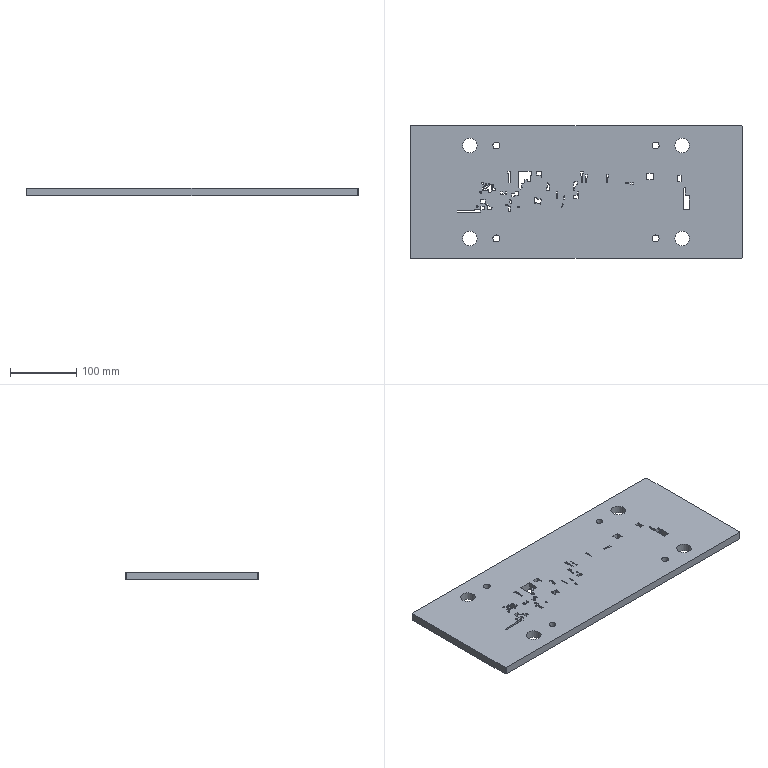Part | NX | features BREP 1 | 1 solid | 359 faces | box 500 x 200 x 12 mm | volume 1158007 mm3 | plane 227 | cylinder 132 | commonest cylinder face diameters 1.2 x65 0.8 x46 3 x4 10.5 x4 22 x4 72.696 x3